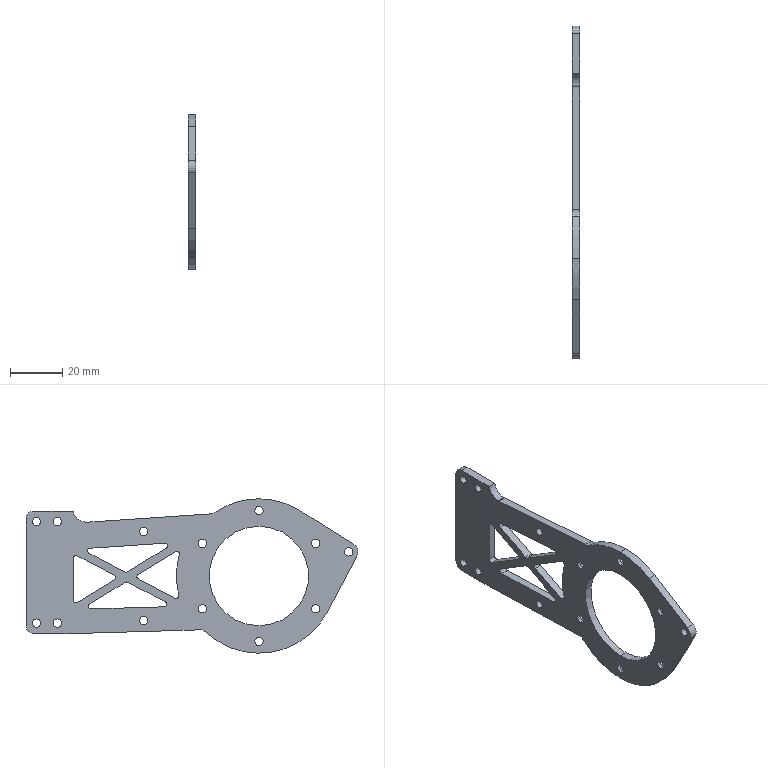Part | SolidWorks | features Fillet 3, ICE 2, Extrusion 1, HoleWzd 1 | 1 solid | 89 faces | box 3 x 126.828 x 59 mm | volume 11105 mm3 | cylinder 57 | plane 20 | cone 12 | commonest cylinder face diameters 3.2 x26 2 x16 6 x5 10 x3 59 x3 38 x2